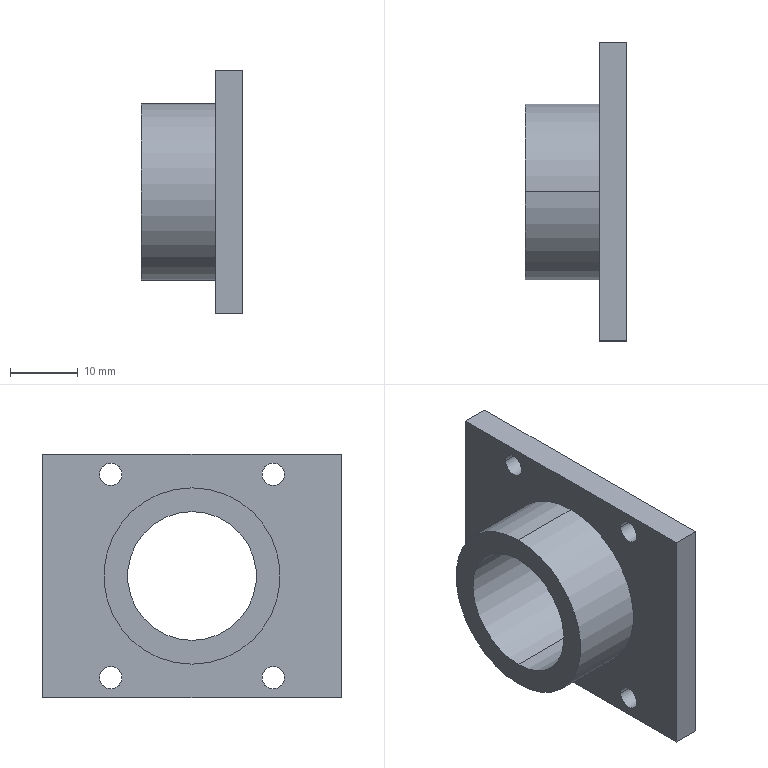Part | SolidWorks | features BaseBody 1 | 1 solid | 19 faces | box 15 x 44 x 36 mm | volume 7786 mm3 | cylinder 12 | plane 7 | commonest cylinder face diameters 3.3 x8 19 x2 26 x2
STEP:
#1=CARTESIAN_POINT('',(-2.,-13.65,33.));
#2=VERTEX_POINT('',#1);
#3=CARTESIAN_POINT('',(-2.,-10.35,33.));
#4=VERTEX_POINT('',#3);
#5=CARTESIAN_POINT('',(-2.,-12.,33.));
#6=DIRECTION('',(1.,0.,0.));
#7=DIRECTION('',(0.,1.,0.));
#8=AXIS2_PLACEMENT_3D('',#5,#6,#7);
#9=CIRCLE('',#8,1.65);
#10=EDGE_CURVE('',#2,#4,#9,.T.);
#11=ORIENTED_EDGE('',*,*,#10,.F.);
#12=CARTESIAN_POINT('',(2.,-13.65,33.));
#13=VERTEX_POINT('',#12);
#14=CARTESIAN_POINT('',(-14.2,-13.65,33.));
#15=DIRECTION('',(1.,0.,0.));
#16=VECTOR('',#15,1000.);
#17=LINE('',#14,#16);
#18=EDGE_CURVE('',#2,#13,#17,.T.);
#19=ORIENTED_EDGE('',*,*,#18,.T.);
#20=CARTESIAN_POINT('',(2.,-10.35,33.));
#21=VERTEX_POINT('',#20);
#22=CARTESIAN_POINT('',(2.,-12.,33.));
#23=DIRECTION('',(-1.,0.,0.));
#24=DIRECTION('',(0.,1.,0.));
#25=AXIS2_PLACEMENT_3D('',#22,#23,#24);
#26=CIRCLE('',#25,1.65);
#27=EDGE_CURVE('',#21,#13,#26,.T.);
#28=ORIENTED_EDGE('',*,*,#27,.F.);
#29=CARTESIAN_POINT('',(-14.2,-10.35,33.));
#30=DIRECTION('',(1.,0.,0.));
#31=VECTOR('',#30,1000.);
#32=LINE('',#29,#31);
#33=EDGE_CURVE('',#4,#21,#32,.T.);
#34=ORIENTED_EDGE('',*,*,#33,.F.);
#35=EDGE_LOOP('',(#11,#19,#28,#34));
#36=FACE_OUTER_BOUND('',#35,.T.);
#37=CARTESIAN_POINT('',(-14.2,-12.,33.));
#38=DIRECTION('',(1.,0.,0.));
#39=DIRECTION('',(0.,1.,0.));
#40=AXIS2_PLACEMENT_3D('',#37,#38,#39);
#41=CYLINDRICAL_SURFACE('',#40,1.65);
#42=ADVANCED_FACE('',(#36),#41,.F.);
#43=CARTESIAN_POINT('',(-2.,-13.65,3.));
#44=VERTEX_POINT('',#43);
#45=CARTESIAN_POINT('',(-2.,-10.35,3.));
#46=VERTEX_POINT('',#45);
#47=CARTESIAN_POINT('',(-2.,-12.,3.));
#48=DIRECTION('',(1.,0.,0.));
#49=DIRECTION('',(0.,1.,0.));
#50=AXIS2_PLACEMENT_3D('',#47,#48,#49);
#51=CIRCLE('',#50,1.65);
#52=EDGE_CURVE('',#44,#46,#51,.T.);
#53=ORIENTED_EDGE('',*,*,#52,.F.);
#54=CARTESIAN_POINT('',(2.,-13.65,3.));
#55=VERTEX_POINT('',#54);
#56=CARTESIAN_POINT('',(-14.2,-13.65,3.));
#57=DIRECTION('',(1.,0.,0.));
#58=VECTOR('',#57,1000.);
#59=LINE('',#56,#58);
#60=EDGE_CURVE('',#44,#55,#59,.T.);
#61=ORIENTED_EDGE('',*,*,#60,.T.);
#62=CARTESIAN_POINT('',(2.,-10.35,3.));
#63=VERTEX_POINT('',#62);
#64=CARTESIAN_POINT('',(2.,-12.,3.));
#65=DIRECTION('',(-1.,0.,0.));
#66=DIRECTION('',(0.,1.,0.));
#67=AXIS2_PLACEMENT_3D('',#64,#65,#66);
#68=CIRCLE('',#67,1.65);
#69=EDGE_CURVE('',#63,#55,#68,.T.);
#70=ORIENTED_EDGE('',*,*,#69,.F.);
#71=CARTESIAN_POINT('',(-14.2,-10.35,3.));
#72=DIRECTION('',(1.,0.,0.));
#73=VECTOR('',#72,1000.);
#74=LINE('',#71,#73);
#75=EDGE_CURVE('',#46,#63,#74,.T.);
#76=ORIENTED_EDGE('',*,*,#75,.F.);
#77=EDGE_LOOP('',(#53,#61,#70,#76));
#78=FACE_OUTER_BOUND('',#77,.T.);
#79=CARTESIAN_POINT('',(-14.2,-12.,3.));
#80=DIRECTION('',(1.,0.,0.));
#81=DIRECTION('',(0.,1.,0.));
#82=AXIS2_PLACEMENT_3D('',#79,#80,#81);
#83=CYLINDRICAL_SURFACE('',#82,1.65);
#84=ADVANCED_FACE('',(#78),#83,.F.);
#85=CARTESIAN_POINT('',(-13.,0.,27.5));
#86=VERTEX_POINT('',#85);
#87=CARTESIAN_POINT('',(-13.,0.,8.5));
#88=VERTEX_POINT('',#87);
#89=CARTESIAN_POINT('',(-13.,0.,18.));
#90=DIRECTION('',(1.,0.,0.));
#91=DIRECTION('',(0.,0.,-1.));
#92=AXIS2_PLACEMENT_3D('',#89,#90,#91);
#93=CIRCLE('',#92,9.5);
#94=EDGE_CURVE('',#86,#88,#93,.T.);
#95=ORIENTED_EDGE('',*,*,#94,.F.);
#96=CARTESIAN_POINT('',(2.,0.,27.5));
#97=VERTEX_POINT('',#96);
#98=CARTESIAN_POINT('',(-3.,0.,27.5));
#99=DIRECTION('',(1.,0.,0.));
#100=VECTOR('',#99,1000.);
#101=LINE('',#98,#100);
#102=EDGE_CURVE('',#86,#97,#101,.T.);
#103=ORIENTED_EDGE('',*,*,#102,.T.);
#104=CARTESIAN_POINT('',(2.,0.,8.5));
#105=VERTEX_POINT('',#104);
#106=CARTESIAN_POINT('',(2.,0.,18.));
#107=DIRECTION('',(-1.,0.,0.));
#108=DIRECTION('',(0.,0.,-1.));
#109=AXIS2_PLACEMENT_3D('',#106,#107,#108);
#110=CIRCLE('',#109,9.5);
#111=EDGE_CURVE('',#105,#97,#110,.T.);
#112=ORIENTED_EDGE('',*,*,#111,.F.);
#113=CARTESIAN_POINT('',(-3.,0.,8.5));
#114=DIRECTION('',(1.,0.,0.));
#115=VECTOR('',#114,1000.);
#116=LINE('',#113,#115);
#117=EDGE_CURVE('',#88,#105,#116,.T.);
#118=ORIENTED_EDGE('',*,*,#117,.F.);
#119=EDGE_LOOP('',(#95,#103,#112,#118));
#120=FACE_OUTER_BOUND('',#119,.T.);
#121=CARTESIAN_POINT('',(-3.,0.,18.));
#122=DIRECTION('',(1.,0.,0.));
#123=DIRECTION('',(0.,0.,-1.));
#124=AXIS2_PLACEMENT_3D('',#121,#122,#123);
#125=CYLINDRICAL_SURFACE('',#124,9.5);
#126=ADVANCED_FACE('',(#120),#125,.F.);
#127=CARTESIAN_POINT('',(-2.,10.35,33.));
#128=VERTEX_POINT('',#127);
#129=CARTESIAN_POINT('',(-2.,13.65,33.));
#130=VERTEX_POINT('',#129);
#131=CARTESIAN_POINT('',(-2.,12.,33.));
#132=DIRECTION('',(1.,0.,0.));
#133=DIRECTION('',(0.,1.,0.));
#134=AXIS2_PLACEMENT_3D('',#131,#132,#133);
#135=CIRCLE('',#134,1.65);
#136=EDGE_CURVE('',#128,#130,#135,.T.);
#137=ORIENTED_EDGE('',*,*,#136,.F.);
#138=CARTESIAN_POINT('',(2.,10.35,33.));
#139=VERTEX_POINT('',#138);
#140=CARTESIAN_POINT('',(-14.2,10.35,33.));
#141=DIRECTION('',(1.,0.,0.));
#142=VECTOR('',#141,1000.);
#143=LINE('',#140,#142);
#144=EDGE_CURVE('',#128,#139,#143,.T.);
#145=ORIENTED_EDGE('',*,*,#144,.T.);
#146=CARTESIAN_POINT('',(2.,13.65,33.));
#147=VERTEX_POINT('',#146);
#148=CARTESIAN_POINT('',(2.,12.,33.));
#149=DIRECTION('',(-1.,0.,0.));
#150=DIRECTION('',(0.,1.,0.));
#151=AXIS2_PLACEMENT_3D('',#148,#149,#150);
#152=CIRCLE('',#151,1.65);
#153=EDGE_CURVE('',#147,#139,#152,.T.);
#154=ORIENTED_EDGE('',*,*,#153,.F.);
#155=CARTESIAN_POINT('',(-14.2,13.65,33.));
#156=DIRECTION('',(1.,0.,0.));
#157=VECTOR('',#156,1000.);
#158=LINE('',#155,#157);
#159=EDGE_CURVE('',#130,#147,#158,.T.);
#160=ORIENTED_EDGE('',*,*,#159,.F.);
#161=EDGE_LOOP('',(#137,#145,#154,#160));
#162=FACE_OUTER_BOUND('',#161,.T.);
#163=CARTESIAN_POINT('',(-14.2,12.,33.));
#164=DIRECTION('',(1.,0.,0.));
#165=DIRECTION('',(0.,1.,0.));
#166=AXIS2_PLACEMENT_3D('',#163,#164,#165);
#167=CYLINDRICAL_SURFACE('',#166,1.65);
#168=ADVANCED_FACE('',(#162),#167,.F.);
#169=CARTESIAN_POINT('',(-2.,10.35,3.));
#170=VERTEX_POINT('',#169);
#171=CARTESIAN_POINT('',(-2.,13.65,3.));
#172=VERTEX_POINT('',#171);
#173=CARTESIAN_POINT('',(-2.,12.,3.));
#174=DIRECTION('',(1.,0.,0.));
#175=DIRECTION('',(0.,1.,0.));
#176=AXIS2_PLACEMENT_3D('',#173,#174,#175);
#177=CIRCLE('',#176,1.65);
#178=EDGE_CURVE('',#170,#172,#177,.T.);
#179=ORIENTED_EDGE('',*,*,#178,.F.);
#180=CARTESIAN_POINT('',(2.,10.35,3.));
#181=VERTEX_POINT('',#180);
#182=CARTESIAN_POINT('',(-14.2,10.35,3.));
#183=DIRECTION('',(1.,0.,0.));
#184=VECTOR('',#183,1000.);
#185=LINE('',#182,#184);
#186=EDGE_CURVE('',#170,#181,#185,.T.);
#187=ORIENTED_EDGE('',*,*,#186,.T.);
#188=CARTESIAN_POINT('',(2.,13.65,3.));
#189=VERTEX_POINT('',#188);
#190=CARTESIAN_POINT('',(2.,12.,3.));
#191=DIRECTION('',(-1.,0.,0.));
#192=DIRECTION('',(0.,1.,0.));
#193=AXIS2_PLACEMENT_3D('',#190,#191,#192);
#194=CIRCLE('',#193,1.65);
#195=EDGE_CURVE('',#189,#181,#194,.T.);
#196=ORIENTED_EDGE('',*,*,#195,.F.);
#197=CARTESIAN_POINT('',(-14.2,13.65,3.));
#198=DIRECTION('',(1.,0.,0.));
#199=VECTOR('',#198,1000.);
#200=LINE('',#197,#199);
#201=EDGE_CURVE('',#172,#189,#200,.T.);
#202=ORIENTED_EDGE('',*,*,#201,.F.);
#203=EDGE_LOOP('',(#179,#187,#196,#202));
#204=FACE_OUTER_BOUND('',#203,.T.);
#205=CARTESIAN_POINT('',(-14.2,12.,3.));
#206=DIRECTION('',(1.,0.,0.));
#207=DIRECTION('',(0.,1.,0.));
#208=AXIS2_PLACEMENT_3D('',#205,#206,#207);
#209=CYLINDRICAL_SURFACE('',#208,1.65);
#210=ADVANCED_FACE('',(#204),#209,.F.);
#211=CARTESIAN_POINT('',(-13.,0.,5.));
#212=VERTEX_POINT('',#211);
#213=CARTESIAN_POINT('',(-13.,0.,31.));
#214=VERTEX_POINT('',#213);
#215=CARTESIAN_POINT('',(-13.,0.,18.));
#216=DIRECTION('',(1.,0.,0.));
#217=DIRECTION('',(0.,0.,-1.));
#218=AXIS2_PLACEMENT_3D('',#215,#216,#217);
#219=CIRCLE('',#218,13.);
#220=EDGE_CURVE('',#212,#214,#219,.T.);
#221=ORIENTED_EDGE('',*,*,#220,.T.);
#222=CARTESIAN_POINT('',(-2.,0.,31.));
#223=VERTEX_POINT('',#222);
#224=CARTESIAN_POINT('',(-13.,0.,31.));
#225=DIRECTION('',(1.,0.,0.));
#226=VECTOR('',#225,1000.);
#227=LINE('',#224,#226);
#228=EDGE_CURVE('',#214,#223,#227,.T.);
#229=ORIENTED_EDGE('',*,*,#228,.T.);
#230=CARTESIAN_POINT('',(-2.,0.,5.));
#231=VERTEX_POINT('',#230);
#232=CARTESIAN_POINT('',(-2.,0.,18.));
#233=DIRECTION('',(-1.,0.,0.));
#234=DIRECTION('',(0.,0.,-1.));
#235=AXIS2_PLACEMENT_3D('',#232,#233,#234);
#236=CIRCLE('',#235,13.);
#237=EDGE_CURVE('',#223,#231,#236,.T.);
#238=ORIENTED_EDGE('',*,*,#237,.T.);
#239=CARTESIAN_POINT('',(-13.,0.,5.));
#240=DIRECTION('',(1.,0.,0.));
#241=VECTOR('',#240,1000.);
#242=LINE('',#239,#241);
#243=EDGE_CURVE('',#212,#231,#242,.T.);
#244=ORIENTED_EDGE('',*,*,#243,.F.);
#245=EDGE_LOOP('',(#221,#229,#238,#244));
#246=FACE_OUTER_BOUND('',#245,.T.);
#247=CARTESIAN_POINT('',(-13.,0.,18.));
#248=DIRECTION('',(1.,0.,0.));
#249=DIRECTION('',(0.,0.,-1.));
#250=AXIS2_PLACEMENT_3D('',#247,#248,#249);
#251=CYLINDRICAL_SURFACE('',#250,13.);
#252=ADVANCED_FACE('',(#246),#251,.T.);
#253=ORIENTED_EDGE('',*,*,#27,.T.);
#254=CARTESIAN_POINT('',(2.,-12.,33.));
#255=DIRECTION('',(-1.,0.,0.));
#256=DIRECTION('',(0.,1.,0.));
#257=AXIS2_PLACEMENT_3D('',#254,#255,#256);
#258=CIRCLE('',#257,1.65);
#259=EDGE_CURVE('',#13,#21,#258,.T.);
#260=ORIENTED_EDGE('',*,*,#259,.T.);
#261=EDGE_LOOP('',(#253,#260));
#262=FACE_BOUND('',#261,.T.);
#263=ORIENTED_EDGE('',*,*,#69,.T.);
#264=CARTESIAN_POINT('',(2.,-12.,3.));
#265=DIRECTION('',(-1.,0.,0.));
#266=DIRECTION('',(0.,1.,0.));
#267=AXIS2_PLACEMENT_3D('',#264,#265,#266);
#268=CIRCLE('',#267,1.65);
#269=EDGE_CURVE('',#55,#63,#268,.T.);
#270=ORIENTED_EDGE('',*,*,#269,.T.);
#271=EDGE_LOOP('',(#263,#270));
#272=FACE_BOUND('',#271,.T.);
#273=ORIENTED_EDGE('',*,*,#111,.T.);
#274=CARTESIAN_POINT('',(2.,0.,18.));
#275=DIRECTION('',(-1.,0.,0.));
#276=DIRECTION('',(0.,0.,-1.));
#277=AXIS2_PLACEMENT_3D('',#274,#275,#276);
#278=CIRCLE('',#277,9.5);
#279=EDGE_CURVE('',#97,#105,#278,.T.);
#280=ORIENTED_EDGE('',*,*,#279,.T.);
#281=EDGE_LOOP('',(#273,#280));
#282=FACE_BOUND('',#281,.T.);
#283=ORIENTED_EDGE('',*,*,#153,.T.);
#284=CARTESIAN_POINT('',(2.,12.,33.));
#285=DIRECTION('',(-1.,0.,0.));
#286=DIRECTION('',(0.,1.,0.));
#287=AXIS2_PLACEMENT_3D('',#284,#285,#286);
#288=CIRCLE('',#287,1.65);
#289=EDGE_CURVE('',#139,#147,#288,.T.);
#290=ORIENTED_EDGE('',*,*,#289,.T.);
#291=EDGE_LOOP('',(#283,#290));
#292=FACE_BOUND('',#291,.T.);
#293=ORIENTED_EDGE('',*,*,#195,.T.);
#294=CARTESIAN_POINT('',(2.,12.,3.));
#295=DIRECTION('',(-1.,0.,0.));
#296=DIRECTION('',(0.,1.,0.));
#297=AXIS2_PLACEMENT_3D('',#294,#295,#296);
#298=CIRCLE('',#297,1.65);
#299=EDGE_CURVE('',#181,#189,#298,.T.);
#300=ORIENTED_EDGE('',*,*,#299,.T.);
#301=EDGE_LOOP('',(#293,#300));
#302=FACE_BOUND('',#301,.T.);
#303=CARTESIAN_POINT('',(2.,22.,0.));
#304=VERTEX_POINT('',#303);
#305=CARTESIAN_POINT('',(2.,22.,36.));
#306=VERTEX_POINT('',#305);
#307=CARTESIAN_POINT('',(2.,22.,0.));
#308=DIRECTION('',(0.,0.,1.));
#309=VECTOR('',#308,1000.);
#310=LINE('',#307,#309);
#311=EDGE_CURVE('',#304,#306,#310,.T.);
#312=ORIENTED_EDGE('',*,*,#311,.T.);
#313=CARTESIAN_POINT('',(2.,-22.,36.));
#314=VERTEX_POINT('',#313);
#315=CARTESIAN_POINT('',(2.,-22.,36.));
#316=DIRECTION('',(0.,-1.,0.));
#317=VECTOR('',#316,1000.);
#318=LINE('',#315,#317);
#319=EDGE_CURVE('',#306,#314,#318,.T.);
#320=ORIENTED_EDGE('',*,*,#319,.T.);
#321=CARTESIAN_POINT('',(2.,-22.,0.));
#322=VERTEX_POINT('',#321);
#323=CARTESIAN_POINT('',(2.,-22.,0.));
#324=DIRECTION('',(0.,0.,-1.));
#325=VECTOR('',#324,1000.);
#326=LINE('',#323,#325);
#327=EDGE_CURVE('',#314,#322,#326,.T.);
#328=ORIENTED_EDGE('',*,*,#327,.T.);
#329=CARTESIAN_POINT('',(2.,-22.,0.));
#330=DIRECTION('',(0.,1.,0.));
#331=VECTOR('',#330,1000.);
#332=LINE('',#329,#331);
#333=EDGE_CURVE('',#322,#304,#332,.T.);
#334=ORIENTED_EDGE('',*,*,#333,.T.);
#335=EDGE_LOOP('',(#312,#320,#328,#334));
#336=FACE_OUTER_BOUND('',#335,.T.);
#337=CARTESIAN_POINT('',(2.,-22.,0.));
#338=DIRECTION('',(1.,0.,0.));
#339=DIRECTION('',(0.,0.,-1.));
#340=AXIS2_PLACEMENT_3D('',#337,#338,#339);
#341=PLANE('',#340);
#342=ADVANCED_FACE('',(#262,#272,#282,#292,#302,#336),#341,.T.);
#343=ORIENTED_EDGE('',*,*,#18,.F.);
#344=CARTESIAN_POINT('',(-2.,-12.,33.));
#345=DIRECTION('',(1.,0.,0.));
#346=DIRECTION('',(0.,1.,0.));
#347=AXIS2_PLACEMENT_3D('',#344,#345,#346);
#348=CIRCLE('',#347,1.65);
#349=EDGE_CURVE('',#4,#2,#348,.T.);
#350=ORIENTED_EDGE('',*,*,#349,.F.);
#351=ORIENTED_EDGE('',*,*,#33,.T.);
#352=ORIENTED_EDGE('',*,*,#259,.F.);
#353=EDGE_LOOP('',(#343,#350,#351,#352));
#354=FACE_OUTER_BOUND('',#353,.T.);
#355=CARTESIAN_POINT('',(-14.2,-12.,33.));
#356=DIRECTION('',(1.,0.,0.));
#357=DIRECTION('',(0.,1.,0.));
#358=AXIS2_PLACEMENT_3D('',#355,#356,#357);
#359=CYLINDRICAL_SURFACE('',#358,1.65);
#360=ADVANCED_FACE('',(#354),#359,.F.);
#361=ORIENTED_EDGE('',*,*,#60,.F.);
#362=CARTESIAN_POINT('',(-2.,-12.,3.));
#363=DIRECTION('',(1.,0.,0.));
#364=DIRECTION('',(0.,1.,0.));
#365=AXIS2_PLACEMENT_3D('',#362,#363,#364);
#366=CIRCLE('',#365,1.65);
#367=EDGE_CURVE('',#46,#44,#366,.T.);
#368=ORIENTED_EDGE('',*,*,#367,.F.);
#369=ORIENTED_EDGE('',*,*,#75,.T.);
#370=ORIENTED_EDGE('',*,*,#269,.F.);
#371=EDGE_LOOP('',(#361,#368,#369,#370));
#372=FACE_OUTER_BOUND('',#371,.T.);
#373=CARTESIAN_POINT('',(-14.2,-12.,3.));
#374=DIRECTION('',(1.,0.,0.));
#375=DIRECTION('',(0.,1.,0.));
#376=AXIS2_PLACEMENT_3D('',#373,#374,#375);
#377=CYLINDRICAL_SURFACE('',#376,1.65);
#378=ADVANCED_FACE('',(#372),#377,.F.);
#379=ORIENTED_EDGE('',*,*,#102,.F.);
#380=CARTESIAN_POINT('',(-13.,0.,18.));
#381=DIRECTION('',(1.,0.,0.));
#382=DIRECTION('',(0.,0.,-1.));
#383=AXIS2_PLACEMENT_3D('',#380,#381,#382);
#384=CIRCLE('',#383,9.5);
#385=EDGE_CURVE('',#88,#86,#384,.T.);
#386=ORIENTED_EDGE('',*,*,#385,.F.);
#387=ORIENTED_EDGE('',*,*,#117,.T.);
#388=ORIENTED_EDGE('',*,*,#279,.F.);
#389=EDGE_LOOP('',(#379,#386,#387,#388));
#390=FACE_OUTER_BOUND('',#389,.T.);
#391=CARTESIAN_POINT('',(-3.,0.,18.));
#392=DIRECTION('',(1.,0.,0.));
#393=DIRECTION('',(0.,0.,-1.));
#394=AXIS2_PLACEMENT_3D('',#391,#392,#393);
#395=CYLINDRICAL_SURFACE('',#394,9.5);
#396=ADVANCED_FACE('',(#390),#395,.F.);
#397=ORIENTED_EDGE('',*,*,#144,.F.);
#398=CARTESIAN_POINT('',(-2.,12.,33.));
#399=DIRECTION('',(1.,0.,0.));
#400=DIRECTION('',(0.,1.,0.));
#401=AXIS2_PLACEMENT_3D('',#398,#399,#400);
#402=CIRCLE('',#401,1.65);
#403=EDGE_CURVE('',#130,#128,#402,.T.);
#404=ORIENTED_EDGE('',*,*,#403,.F.);
#405=ORIENTED_EDGE('',*,*,#159,.T.);
#406=ORIENTED_EDGE('',*,*,#289,.F.);
#407=EDGE_LOOP('',(#397,#404,#405,#406));
#408=FACE_OUTER_BOUND('',#407,.T.);
#409=CARTESIAN_POINT('',(-14.2,12.,33.));
#410=DIRECTION('',(1.,0.,0.));
#411=DIRECTION('',(0.,1.,0.));
#412=AXIS2_PLACEMENT_3D('',#409,#410,#411);
#413=CYLINDRICAL_SURFACE('',#412,1.65);
#414=ADVANCED_FACE('',(#408),#413,.F.);
#415=ORIENTED_EDGE('',*,*,#186,.F.);
#416=CARTESIAN_POINT('',(-2.,12.,3.));
#417=DIRECTION('',(1.,0.,0.));
#418=DIRECTION('',(0.,1.,0.));
#419=AXIS2_PLACEMENT_3D('',#416,#417,#418);
#420=CIRCLE('',#419,1.65);
#421=EDGE_CURVE('',#172,#170,#420,.T.);
#422=ORIENTED_EDGE('',*,*,#421,.F.);
#423=ORIENTED_EDGE('',*,*,#201,.T.);
#424=ORIENTED_EDGE('',*,*,#299,.F.);
#425=EDGE_LOOP('',(#415,#422,#423,#424));
#426=FACE_OUTER_BOUND('',#425,.T.);
#427=CARTESIAN_POINT('',(-14.2,12.,3.));
#428=DIRECTION('',(1.,0.,0.));
#429=DIRECTION('',(0.,1.,0.));
#430=AXIS2_PLACEMENT_3D('',#427,#428,#429);
#431=CYLINDRICAL_SURFACE('',#430,1.65);
#432=ADVANCED_FACE('',(#426),#431,.F.);
#433=ORIENTED_EDGE('',*,*,#319,.F.);
#434=CARTESIAN_POINT('',(-2.,22.,36.));
#435=VERTEX_POINT('',#434);
#436=CARTESIAN_POINT('',(-2.,22.,36.));
#437=DIRECTION('',(-1.,0.,0.));
#438=VECTOR('',#437,1000.);
#439=LINE('',#436,#438);
#440=EDGE_CURVE('',#306,#435,#439,.T.);
#441=ORIENTED_EDGE('',*,*,#440,.T.);
#442=CARTESIAN_POINT('',(-2.,-22.,36.));
#443=VERTEX_POINT('',#442);
#444=CARTESIAN_POINT('',(-2.,-22.,36.));
#445=DIRECTION('',(0.,-1.,0.));
#446=VECTOR('',#445,1000.);
#447=LINE('',#444,#446);
#448=EDGE_CURVE('',#435,#443,#447,.T.);
#449=ORIENTED_EDGE('',*,*,#448,.T.);
#450=CARTESIAN_POINT('',(-2.,-22.,36.));
#451=DIRECTION('',(1.,0.,0.));
#452=VECTOR('',#451,1000.);
#453=LINE('',#450,#452);
#454=EDGE_CURVE('',#443,#314,#453,.T.);
#455=ORIENTED_EDGE('',*,*,#454,.T.);
#456=EDGE_LOOP('',(#433,#441,#449,#455));
#457=FACE_OUTER_BOUND('',#456,.T.);
#458=CARTESIAN_POINT('',(-2.,-22.,36.));
#459=DIRECTION('',(0.,0.,1.));
#460=DIRECTION('',(1.,0.,0.));
#461=AXIS2_PLACEMENT_3D('',#458,#459,#460);
#462=PLANE('',#461);
#463=ADVANCED_FACE('',(#457),#462,.T.);
#464=ORIENTED_EDGE('',*,*,#440,.F.);
#465=ORIENTED_EDGE('',*,*,#311,.F.);
#466=CARTESIAN_POINT('',(-2.,22.,0.));
#467=VERTEX_POINT('',#466);
#468=CARTESIAN_POINT('',(-2.,22.,0.));
#469=DIRECTION('',(-1.,0.,0.));
#470=VECTOR('',#469,1000.);
#471=LINE('',#468,#470);
#472=EDGE_CURVE('',#304,#467,#471,.T.);
#473=ORIENTED_EDGE('',*,*,#472,.T.);
#474=CARTESIAN_POINT('',(-2.,22.,0.));
#475=DIRECTION('',(0.,0.,1.));
#476=VECTOR('',#475,1000.);
#477=LINE('',#474,#476);
#478=EDGE_CURVE('',#467,#435,#477,.T.);
#479=ORIENTED_EDGE('',*,*,#478,.T.);
#480=EDGE_LOOP('',(#464,#465,#473,#479));
#481=FACE_OUTER_BOUND('',#480,.T.);
#482=CARTESIAN_POINT('',(-2.,22.,0.));
#483=DIRECTION('',(0.,1.,0.));
#484=DIRECTION('',(0.,0.,1.));
#485=AXIS2_PLACEMENT_3D('',#482,#483,#484);
#486=PLANE('',#485);
#487=ADVANCED_FACE('',(#481),#486,.T.);
#488=ORIENTED_EDGE('',*,*,#333,.F.);
#489=CARTESIAN_POINT('',(-2.,-22.,0.));
#490=VERTEX_POINT('',#489);
#491=CARTESIAN_POINT('',(-2.,-22.,0.));
#492=DIRECTION('',(1.,0.,0.));
#493=VECTOR('',#492,1000.);
#494=LINE('',#491,#493);
#495=EDGE_CURVE('',#490,#322,#494,.T.);
#496=ORIENTED_EDGE('',*,*,#495,.F.);
#497=CARTESIAN_POINT('',(-2.,-22.,0.));
#498=DIRECTION('',(0.,-1.,0.));
#499=VECTOR('',#498,1000.);
#500=LINE('',#497,#499);
#501=EDGE_CURVE('',#467,#490,#500,.T.);
#502=ORIENTED_EDGE('',*,*,#501,.F.);
#503=ORIENTED_EDGE('',*,*,#472,.F.);
#504=EDGE_LOOP('',(#488,#496,#502,#503));
#505=FACE_OUTER_BOUND('',#504,.T.);
#506=CARTESIAN_POINT('',(-2.,-22.,0.));
#507=DIRECTION('',(0.,0.,1.));
#508=DIRECTION('',(1.,0.,0.));
#509=AXIS2_PLACEMENT_3D('',#506,#507,#508);
#510=PLANE('',#509);
#511=ADVANCED_FACE('',(#505),#510,.F.);
#512=ORIENTED_EDGE('',*,*,#454,.F.);
#513=CARTESIAN_POINT('',(-2.,-22.,0.));
#514=DIRECTION('',(0.,0.,1.));
#515=VECTOR('',#514,1000.);
#516=LINE('',#513,#515);
#517=EDGE_CURVE('',#490,#443,#516,.T.);
#518=ORIENTED_EDGE('',*,*,#517,.F.);
#519=ORIENTED_EDGE('',*,*,#495,.T.);
#520=ORIENTED_EDGE('',*,*,#327,.F.);
#521=EDGE_LOOP('',(#512,#518,#519,#520));
#522=FACE_OUTER_BOUND('',#521,.T.);
#523=CARTESIAN_POINT('',(-2.,-22.,0.));
#524=DIRECTION('',(0.,1.,0.));
#525=DIRECTION('',(0.,0.,1.));
#526=AXIS2_PLACEMENT_3D('',#523,#524,#525);
#527=PLANE('',#526);
#528=ADVANCED_FACE('',(#522),#527,.F.);
#529=ORIENTED_EDGE('',*,*,#349,.T.);
#530=ORIENTED_EDGE('',*,*,#10,.T.);
#531=EDGE_LOOP('',(#529,#530));
#532=FACE_BOUND('',#531,.T.);
#533=ORIENTED_EDGE('',*,*,#367,.T.);
#534=ORIENTED_EDGE('',*,*,#52,.T.);
#535=EDGE_LOOP('',(#533,#534));
#536=FACE_BOUND('',#535,.T.);
#537=CARTESIAN_POINT('',(-2.,0.,18.));
#538=DIRECTION('',(-1.,0.,0.));
#539=DIRECTION('',(0.,0.,-1.));
#540=AXIS2_PLACEMENT_3D('',#537,#538,#539);
#541=CIRCLE('',#540,13.);
#542=EDGE_CURVE('',#231,#223,#541,.T.);
#543=ORIENTED_EDGE('',*,*,#542,.F.);
#544=ORIENTED_EDGE('',*,*,#237,.F.);
#545=EDGE_LOOP('',(#543,#544));
#546=FACE_BOUND('',#545,.T.);
#547=ORIENTED_EDGE('',*,*,#403,.T.);
#548=ORIENTED_EDGE('',*,*,#136,.T.);
#549=EDGE_LOOP('',(#547,#548));
#550=FACE_BOUND('',#549,.T.);
#551=ORIENTED_EDGE('',*,*,#421,.T.);
#552=ORIENTED_EDGE('',*,*,#178,.T.);
#553=EDGE_LOOP('',(#551,#552));
#554=FACE_BOUND('',#553,.T.);
#555=ORIENTED_EDGE('',*,*,#478,.F.);
#556=ORIENTED_EDGE('',*,*,#501,.T.);
#557=ORIENTED_EDGE('',*,*,#517,.T.);
#558=ORIENTED_EDGE('',*,*,#448,.F.);
#559=EDGE_LOOP('',(#555,#556,#557,#558));
#560=FACE_OUTER_BOUND('',#559,.T.);
#561=CARTESIAN_POINT('',(-2.,-22.,0.));
#562=DIRECTION('',(1.,0.,0.));
#563=DIRECTION('',(0.,0.,-1.));
#564=AXIS2_PLACEMENT_3D('',#561,#562,#563);
#565=PLANE('',#564);
#566=ADVANCED_FACE('',(#532,#536,#546,#550,#554,#560),#565,.F.);
#567=ORIENTED_EDGE('',*,*,#385,.T.);
#568=ORIENTED_EDGE('',*,*,#94,.T.);
#569=EDGE_LOOP('',(#567,#568));
#570=FACE_BOUND('',#569,.T.);
#571=ORIENTED_EDGE('',*,*,#220,.F.);
#572=CARTESIAN_POINT('',(-13.,0.,18.));
#573=DIRECTION('',(1.,0.,0.));
#574=DIRECTION('',(0.,0.,-1.));
#575=AXIS2_PLACEMENT_3D('',#572,#573,#574);
#576=CIRCLE('',#575,13.);
#577=EDGE_CURVE('',#214,#212,#576,.T.);
#578=ORIENTED_EDGE('',*,*,#577,.F.);
#579=EDGE_LOOP('',(#571,#578));
#580=FACE_OUTER_BOUND('',#579,.T.);
#581=CARTESIAN_POINT('',(-13.,0.,18.));
#582=DIRECTION('',(1.,0.,0.));
#583=DIRECTION('',(0.,0.,-1.));
#584=AXIS2_PLACEMENT_3D('',#581,#582,#583);
#585=PLANE('',#584);
#586=ADVANCED_FACE('',(#570,#580),#585,.F.);
#587=ORIENTED_EDGE('',*,*,#228,.F.);
#588=ORIENTED_EDGE('',*,*,#577,.T.);
#589=ORIENTED_EDGE('',*,*,#243,.T.);
#590=ORIENTED_EDGE('',*,*,#542,.T.);
#591=EDGE_LOOP('',(#587,#588,#589,#590));
#592=FACE_OUTER_BOUND('',#591,.T.);
#593=CARTESIAN_POINT('',(-13.,0.,18.));
#594=DIRECTION('',(1.,0.,0.));
#595=DIRECTION('',(0.,0.,-1.));
#596=AXIS2_PLACEMENT_3D('',#593,#594,#595);
#597=CYLINDRICAL_SURFACE('',#596,13.);
#598=ADVANCED_FACE('',(#592),#597,.T.);
#599=CLOSED_SHELL('',(#42,#84,#126,#168,#210,#252,#342,#360,#378,#396,#414,#432,#463,#487,#511,#528,#566,#586,#598));
#600=MANIFOLD_SOLID_BREP('',#599);
#601=CARTESIAN_POINT('',(0.,0.,0.));
#602=DIRECTION('',(0.,0.,1.));
#603=DIRECTION('',(1.,0.,0.));
#604=AXIS2_PLACEMENT_3D('',#601,#602,#603);
#605=(LENGTH_UNIT()NAMED_UNIT(*)SI_UNIT(.MILLI.,.METRE.));
#606=UNCERTAINTY_MEASURE_WITH_UNIT(LENGTH_MEASURE(0.00001),#605,'','');
#607=(NAMED_UNIT(*)PLANE_ANGLE_UNIT()SI_UNIT($,.RADIAN.));
#608=(NAMED_UNIT(*)SI_UNIT($,.STERADIAN.)SOLID_ANGLE_UNIT());
#609=(GEOMETRIC_REPRESENTATION_CONTEXT(3)GLOBAL_UNCERTAINTY_ASSIGNED_CONTEXT((#606))GLOBAL_UNIT_ASSIGNED_CONTEXT((#605,#607,#608))REPRESENTATION_CONTEXT('',''));
#610=ADVANCED_BREP_SHAPE_REPRESENTATION('',(#600,#604),#609);